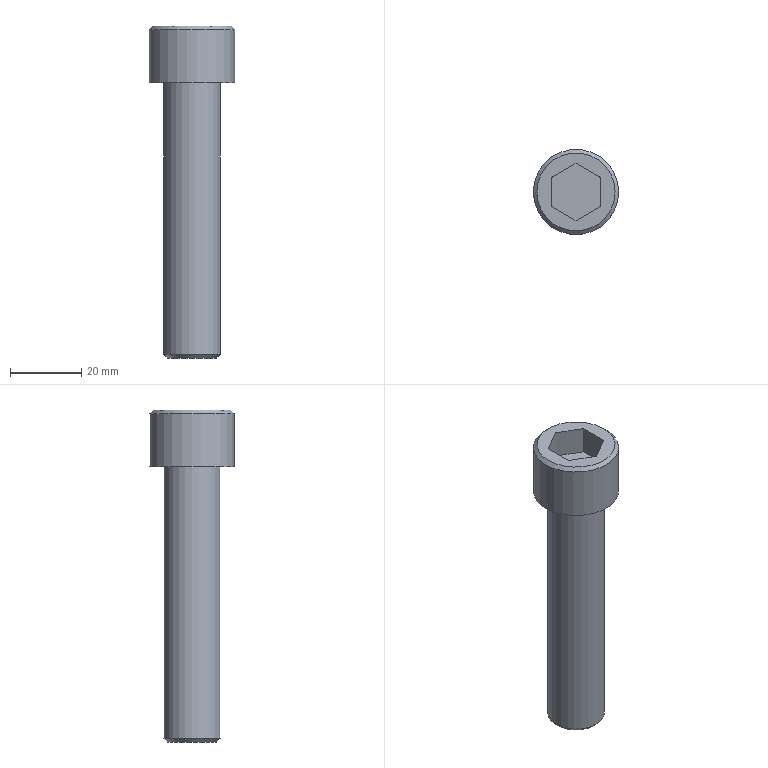Part | STEP file | M16.00-95.00 | 1 solid | 14 faces | box 24 x 24 x 93.469 mm | volume 21396 mm3 | plane 10 | cylinder 2 | cone 2 | commonest cylinder face diameters 16 x1 24 x1